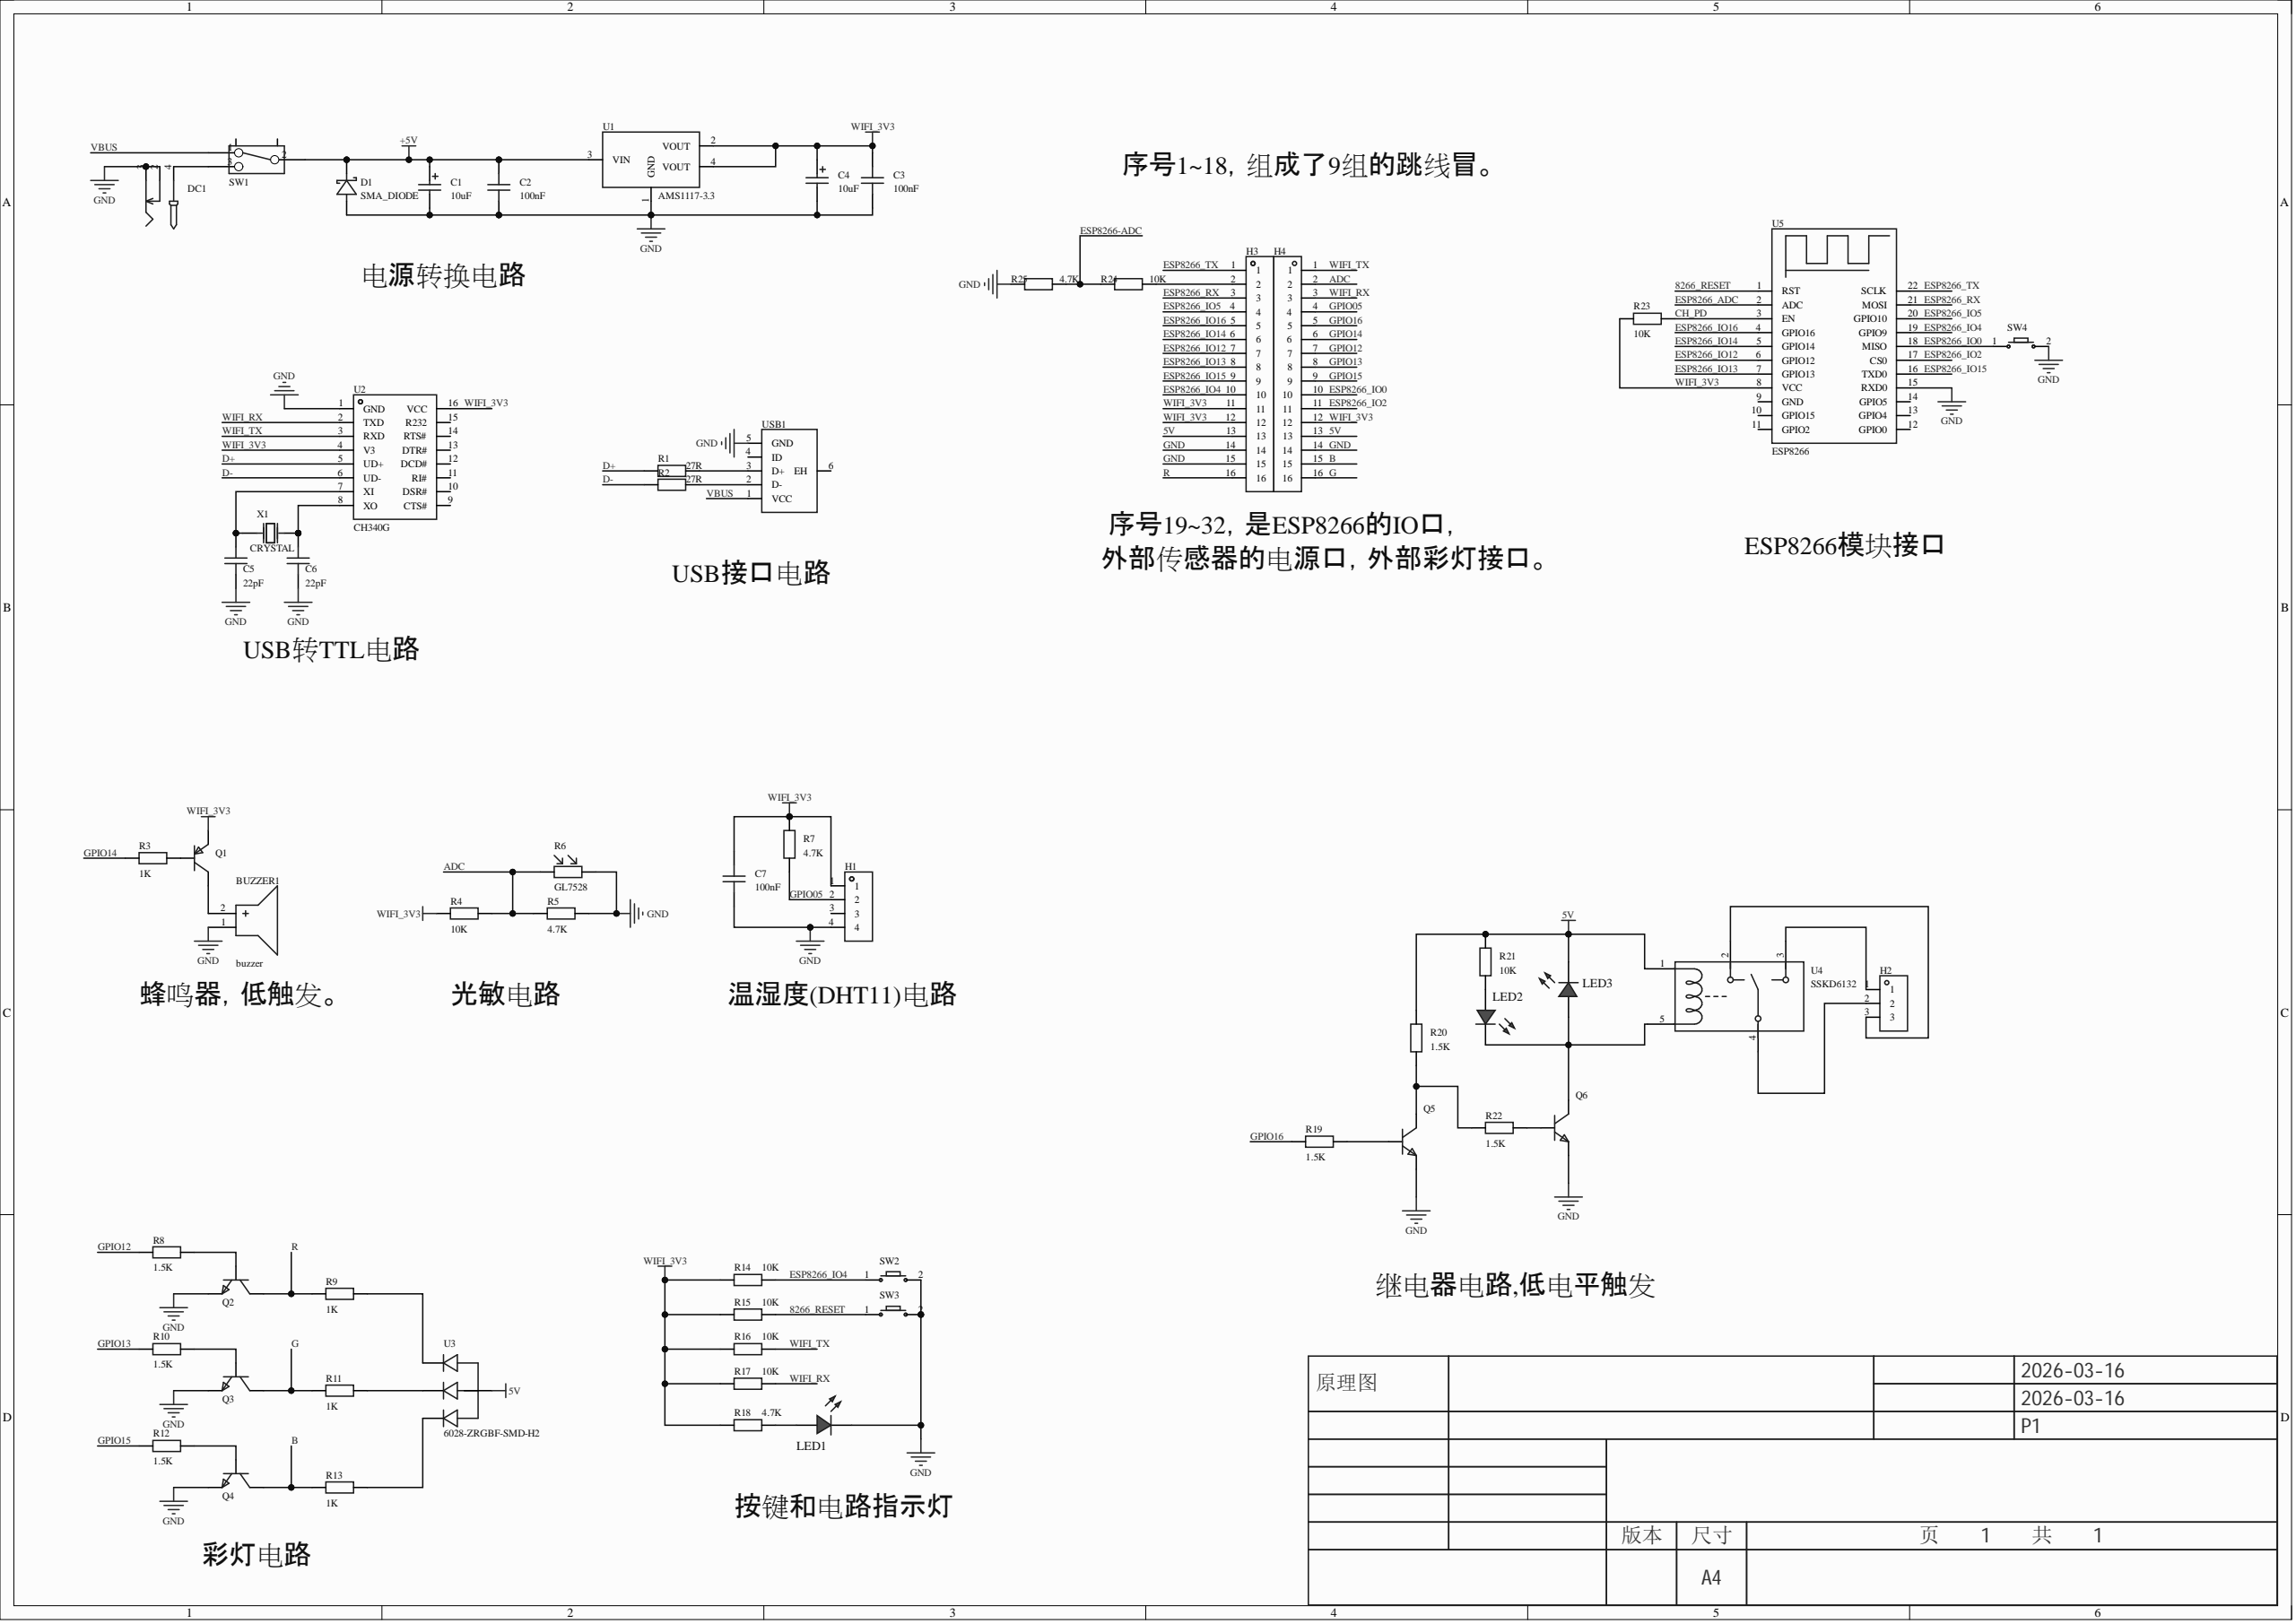Circuit board | Altium Designer | 59 parts | 56 nets
Bill of materials:
Comment,Description,Designator,Footprint,LibRef,Quantity
"buzzer","","BUZZER1","BUZ-TH_BD12.0-P6.00-D0.9-RD","buzzer","1"
"10uF","","C1, C4","C_Ele_SMD_5x5.4mm","C_Ele_SMD_5x5.4mm","2"
"100nF","","C2, C3, C7","C0603","CAP_0603","3"
"22pF","","C5, C6","C0603","CAP_0603","2"
"SMA_DIODE","","D1","SOD-57_BD3.8-L4.6-P9.00-D0.8-RD","SMA_DIODE","1"
"","","DC1","DC-2.0","DC-005_2.0","1"
"","","H1","HDR-TH_4P-P2.54-V-F","HDR-F_2.54_1x4P","1"
"","","H2","HDR-TH_3P-P2.54-V-F","HDR-F_2.54_1x3P","1"
"","","H3, H4","HDR-TH_16P-P2.54-V-F","HDR-F_2.54_1x16P","2"
"","","LED1, LED2, LED3","LED_0805","LED_0805-R","3"
"","","Q1","S8550P_SOT","S8550_SOT_PNP","1"
"","","Q2, Q3, Q4, Q5, Q6","S8050_SOT-23","S8050_SOT_NPN","5"
"27R","","R1, R2","R0603","Res_0603","2"
"1K","","R3, R9, R11, R13","R0805","Res_0805","4"
"10K","","R4, R14, R15, R16, R17, R21, R23","R0805","Res_0805","7"
"4.7K","","R5, R7, R18","R0805","Res_0805","3"
"GL7528","暗电阻:-;光谱峰值(波长):-;","R6","RES-TH_L7.0-W5.9-P5.00-D0.5","GL7528","1"
"1.5K","","R8, R10, R12, R19, R20, R22","R0805","Res_0805","6"
"10K","","R24","Res_1/8W","Res_AXIAL-1/8W","1"
"4.7K","","R25","Res_1/8W","Res_AXIAL-1/8W","1"
"","","SW1","拨动开关_侧","拨动开关_侧","1"
"","","SW2, SW3, SW4","Key_SMD_3x4x2","Key_SMD_3x4x2","3"
"AMS1117-3.3","输出类型:固定;工作电压:16V;输出电压:3.3V;输出电流:1A;电源纹波抑制比(PSRR):72dB@(120Hz);输出极性:正极;","U1","SOT-223-3_L6.5-W3.4-P2.30-LS7.0-BR","AMS1117-3.3_C6186","1"
"CH340G","应用功能:USB转UART;接口协议:USB 2.0;数据速率:2Mbps;","U2","SOIC-16_L9.9-W3.9-P1.27-LS6.0-BL","CH340G","1"
"6028-ZRGBF-SMD-H2","","U3","LED-SMD_4P-L3.2-W2.8_ZRGBF-SMD-H2","6028-ZRGBF-SMD-H2","1"
"SSKD6132","","U4","RELAY-TH_G2R-1","SSKD6132","1"
"ESP8266","","U5","WIFIM-SMD_ESP-12F-ESP8266MOD","ESP8266","1"
"","","USB1","USB_Micro","USB_Micro-B","1"
"CRYSTAL","晶振类型:贴片晶振;频率:8MHz;常温频差:±10ppm;负载电容:20pF;频率稳定度:±20ppm;","X1","CRYSTAL-SMD_L5.0-W3.2","X50328MSB2GI","1"
Netlist (Protel format):
[
BUZZER1
BUZ-TH_BD12.0-P6.00-D0.9-RD
buzzer



]
[
C1
C_Ele_SMD_5x5.4mm
10uF



]
[
C2
C0603
100nF



]
[
C3
C0603
100nF



]
[
C4
C_Ele_SMD_5x5.4mm
10uF



]
[
C5
C0603
22pF



]
[
C6
C0603
22pF



]
[
C7
C0603
100nF



]
[
D1
SOD-57_BD3.8-L4.6-P9.00-D0.8-RD
SMA_DIODE



]
[
DC1
DC-2.0




]
[
H1
HDR-TH_4P-P2.54-V-F




]
[
H2
HDR-TH_3P-P2.54-V-F




]
[
H3
HDR-TH_16P-P2.54-V-F




]
[
H4
HDR-TH_16P-P2.54-V-F




]
[
LED1
LED_0805




]
[
LED2
LED_0805




]
[
LED3
LED_0805




]
[
Q1
S8550P_SOT




]
[
Q2
S8050_SOT-23




]
[
Q3
S8050_SOT-23




]
[
Q4
S8050_SOT-23




]
[
Q5
S8050_SOT-23




]
[
Q6
S8050_SOT-23




]
[
R1
R0603
27R



]
[
R2
R0603
27R



]
[
R3
R0805
1K



]
[
R4
R0805
10K



]
[
R5
R0805
4.7K



]
[
R6
RES-TH_L7.0-W5.9-P5.00-D0.5
GL7528



]
[
R7
R0805
4.7K



]
[
R8
R0805
1.5K



]
[
R9
R0805
1K



]
[
R10
R0805
1.5K



]
[
R11
R0805
1K



]
[
R12
R0805
1.5K



]
[
R13
R0805
1K



]
[
R14
R0805
10K



]
[
R15
R0805
10K



]
[
R16
R0805
10K



]
[
R17
R0805
10K



]
[
R18
R0805
4.7K



]
[
R19
R0805
1.5K



]
[
R20
R0805
1.5K



]
[
R21
R0805
10K



]
[
R22
R0805
1.5K



]
[
R23
R0805
10K



]
[
R24
Res_1/8W
10K



]
[
R25
Res_1/8W
4.7K



]
[
SW1
拨动开关_侧




]
[
SW2
Key_SMD_3x4x2




]
[
SW3
Key_SMD_3x4x2




]
[
SW4
Key_SMD_3x4x2




]
[
U1
SOT-223-3_L6.5-W3.4-P2.30-LS7.0-BR
AMS1117-3.3



]
[
U2
SOIC-16_L9.9-W3.9-P1.27-LS6.0-BL
CH340G



]
[
U3
LED-SMD_4P-L3.2-W2.8_ZRGBF-SMD-H2
6028-ZRGBF-SMD-H2



]
[
U4
RELAY-TH_G2R-1
SSKD6132



]
[
U5
WIFIM-SMD_ESP-12F-ESP8266MOD
ESP8266



]
[
USB1
USB_Micro




]
[
X1
CRYSTAL-SMD_L5.0-W3.2
CRYSTAL



]
(
WIFI_TX
H4-1
R16-2
U2-3
)
(
WIFI_RX
H4-3
R17-2
U2-2
)
(
WIFI_3V3
C3-2
C4-1
C7-2
H1-1
H3-11
H3-12
H4-12
Q1-2
R4-1
R7-2
R14-1
R15-1
R16-1
R17-1
R18-1
R23-1
U1-2
U1-4
U2-4
U2-16
U5-8
)
(
VBUS
SW1-1
USB1-1
)
(
R
H3-16
Q2-3
R9-1
)
(
NetR13_2
R13-2
U3-3
)
(
NetR11_2
R11-2
U3-4
)
(
NetR9_2
R9-2
U3-1
)
(
NetR2_2
R2-2
USB1-2
)
(
NetR1_2
R1-2
USB1-3
)
(
NetQ6_1
Q6-1
R22-2
)
(
NetQ5_3
Q5-3
R20-1
R22-1
)
(
NetQ5_1
Q5-1
R19-2
)
(
NetQ4_1
Q4-1
R12-2
)
(
NetQ3_1
Q3-1
R10-2
)
(
NetQ2_1
Q2-1
R8-2
)
(
NetQ1_1
Q1-1
R3-2
)
(
NetLED2_2
LED2-2
R21-1
)
(
NetLED2_1
LED2-1
LED3-2
Q6-3
U4-5
)
(
NetLED1_2
LED1-2
R18-2
)
(
NetH3_2
H3-2
R24-2
)
(
NetH2_3
H2-3
U4-2
)
(
NetH2_2
H2-2
U4-4
)
(
NetH2_1
H2-1
U4-3
)
(
NetDC1_4
DC1-4
SW1-3
)
(
NetC6_2
C6-2
U2-8
X1-2
)
(
NetC5_2
C5-2
U2-7
X1-1
)
(
NetBUZZER1_2
BUZZER1-2
Q1-3
)
(
GPIO16
H4-5
R19-1
)
(
GPIO15
H4-9
R12-1
)
(
GPIO14
H4-6
R3-1
)
(
GPIO13
H4-8
R10-1
)
(
GPIO12
H4-7
R8-1
)
(
GPIO05
H1-2
H4-4
R7-1
)
(
GND
BUZZER1-1
C1-2
C2-1
C3-1
C4-2
C5-1
C6-1
C7-1
D1-2
DC1-2
DC1-3
H1-4
H3-14
H3-15
H4-14
LED1-1
Q2-2
Q3-2
Q4-2
Q5-2
Q6-2
R5-2
R6-2
R25-1
SW2-2
SW3-2
SW4-2
U1-1
U2-1
U5-15
USB1-5
)
(
G
H4-16
Q3-3
R11-1
)
(
ESP8266_TX
H3-1
U5-22
)
(
ESP8266_RX
H3-3
U5-21
)
(
ESP8266_IO16
H3-5
U5-4
)
(
ESP8266_IO15
H3-9
U5-16
)
(
ESP8266_IO14
H3-6
U5-5
)
(
ESP8266_IO13
H3-8
U5-7
)
(
ESP8266_IO12
H3-7
U5-6
)
(
ESP8266_IO5
H3-4
U5-20
)
(
ESP8266_IO4
H3-10
R14-2
SW2-1
U5-19
)
(
ESP8266_IO2
H4-11
U5-17
)
(
ESP8266_IO0
H4-10
SW4-1
U5-18
)
(
ESP8266-ADC
R24-1
R25-2
)
(
D-
R2-1
U2-6
)
(
D+
R1-1
U2-5
)
(
CH_PD
R23-2
U5-3
)
(
B
H4-15
Q4-3
R13-1
)
(
ADC
H4-2
R4-2
R5-1
R6-1
)
(
+5V
C1-1
C2-2
D1-1
SW1-2
U1-3
)
(
8266_RESET
R15-2
SW3-1
U5-1
)
(
5V
H3-13
H4-13
LED3-1
R20-2
R21-2
U3-2
U4-1
)